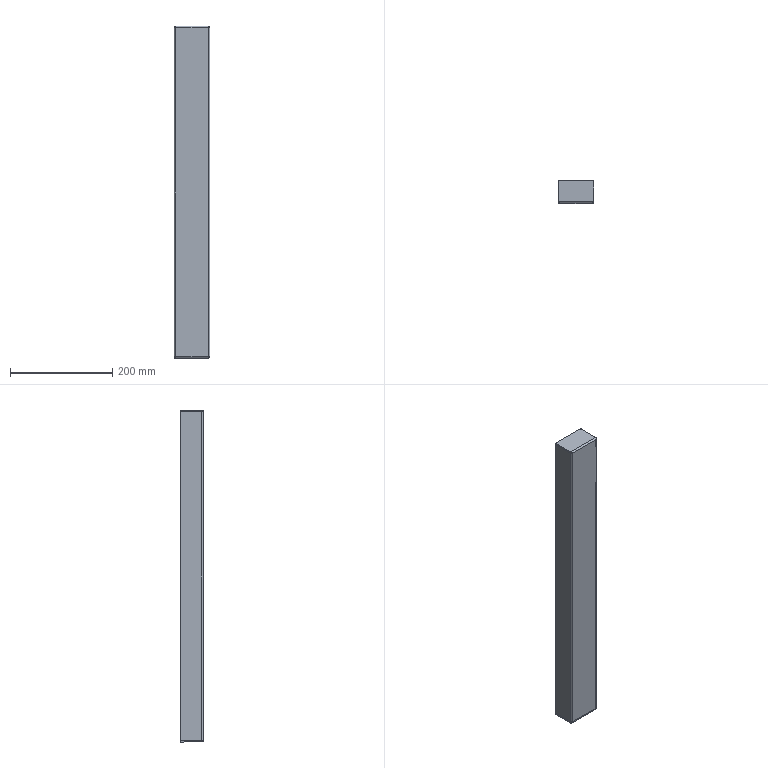Part | SolidWorks | 1 solid | 56 faces | box 70 x 45 x 650 mm | volume 334042 mm3 | plane 36 | cylinder 16 | spline 4 | commonest cylinder face diameters 0.2 x5 6.2 x5 13 x4 6 x2